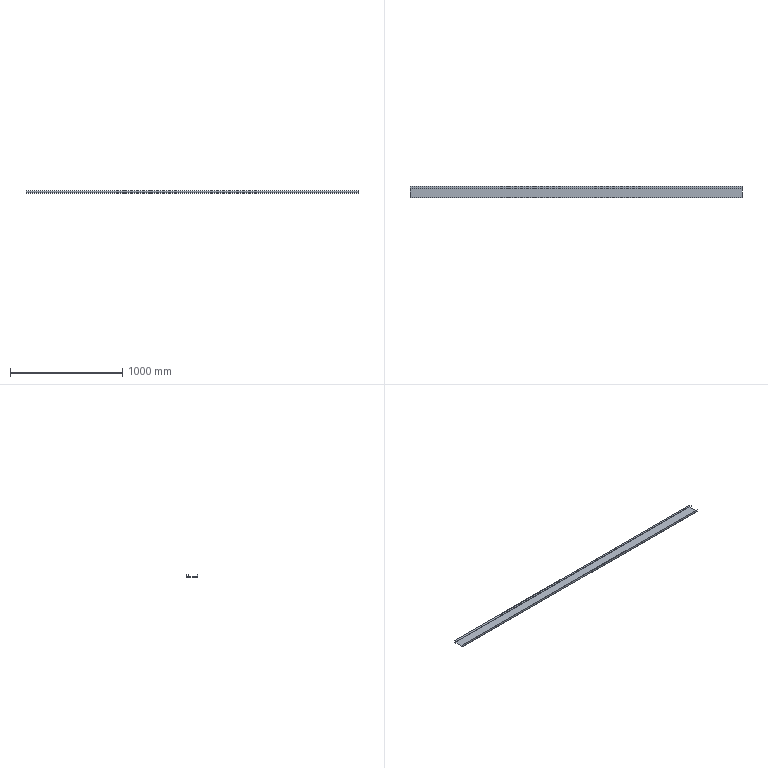Part | STEP file | 粉仓楼梯通道护栏1踢脚Plate | 1 solid | 18 faces | box 2960 x 100 x 20 mm | volume 680415 mm3 | plane 12 | cylinder 6 | commonest cylinder face diameters 2 x3 5 x3
STEP:
#1=CARTESIAN_POINT('',(0.,0.,0.));
#2=DIRECTION('',(0.,0.,1.));
#3=DIRECTION('',(1.,0.,0.));
#4=AXIS2_PLACEMENT_3D('',#1,#2,#3);
#5=CARTESIAN_POINT('',(-1480.,1.5,2.5));
#6=VERTEX_POINT('',#5);
#7=CARTESIAN_POINT('',(-1480.,1.5,20.));
#8=VERTEX_POINT('',#7);
#9=CARTESIAN_POINT('',(-1480.,1.5,2.5));
#10=DIRECTION('',(0.,0.,1.));
#11=VECTOR('',#10,1.);
#12=LINE('',#9,#11);
#13=CARTESIAN_POINT('',(1480.,1.5,2.5));
#14=DIRECTION('',(0.,-1.,0.));
#15=DIRECTION('',(0.,0.,-1.));
#16=AXIS2_PLACEMENT_3D('',#13,#14,#15);
#17=PLANE('',#16);
#18=CARTESIAN_POINT('',(0.,-2960.));
#19=DIRECTION('',(-1.,0.));
#20=VECTOR('',#19,1.);
#21=LINE('',#18,#20);
#22=(GEOMETRIC_REPRESENTATION_CONTEXT(2)PARAMETRIC_REPRESENTATION_CONTEXT()REPRESENTATION_CONTEXT('',''));
#23=DEFINITIONAL_REPRESENTATION('',(#21),#22);
#24=PCURVE('',#17,#23);
#25=CARTESIAN_POINT('',(-1480.,2.5,2.5));
#26=DIRECTION('',(-1.,0.,0.));
#27=DIRECTION('',(0.,0.,1.));
#28=AXIS2_PLACEMENT_3D('',#25,#26,#27);
#29=PLANE('',#28);
#30=CARTESIAN_POINT('',(0.,-1.));
#31=DIRECTION('',(1.,0.));
#32=VECTOR('',#31,1.);
#33=LINE('',#30,#32);
#34=(GEOMETRIC_REPRESENTATION_CONTEXT(2)PARAMETRIC_REPRESENTATION_CONTEXT()REPRESENTATION_CONTEXT('',''));
#35=DEFINITIONAL_REPRESENTATION('',(#33),#34);
#36=PCURVE('',#29,#35);
#37=SURFACE_CURVE('',#12,(#24,#36),.PCURVE_S1.);
#38=EDGE_CURVE('',#6,#8,#37,.T.);
#39=ORIENTED_EDGE('',*,*,#38,.T.);
#40=CARTESIAN_POINT('',(1480.,1.5,20.));
#41=VERTEX_POINT('',#40);
#42=CARTESIAN_POINT('',(1480.,1.5,20.));
#43=DIRECTION('',(-1.,0.,0.));
#44=VECTOR('',#43,1.);
#45=LINE('',#42,#44);
#46=CARTESIAN_POINT('',(-17.5,0.));
#47=DIRECTION('',(0.,-1.));
#48=VECTOR('',#47,1.);
#49=LINE('',#46,#48);
#50=(GEOMETRIC_REPRESENTATION_CONTEXT(2)PARAMETRIC_REPRESENTATION_CONTEXT()REPRESENTATION_CONTEXT('',''));
#51=DEFINITIONAL_REPRESENTATION('',(#49),#50);
#52=PCURVE('',#17,#51);
#53=CARTESIAN_POINT('',(1480.,0.,20.));
#54=DIRECTION('',(0.,0.,1.));
#55=DIRECTION('',(1.,0.,0.));
#56=AXIS2_PLACEMENT_3D('',#53,#54,#55);
#57=PLANE('',#56);
#58=CARTESIAN_POINT('',(0.,1.5));
#59=DIRECTION('',(-1.,0.));
#60=VECTOR('',#59,1.);
#61=LINE('',#58,#60);
#62=(GEOMETRIC_REPRESENTATION_CONTEXT(2)PARAMETRIC_REPRESENTATION_CONTEXT()REPRESENTATION_CONTEXT('',''));
#63=DEFINITIONAL_REPRESENTATION('',(#61),#62);
#64=PCURVE('',#57,#63);
#65=SURFACE_CURVE('',#45,(#52,#64),.PCURVE_S1.);
#66=EDGE_CURVE('',#41,#8,#65,.T.);
#67=ORIENTED_EDGE('',*,*,#66,.F.);
#68=CARTESIAN_POINT('',(1480.,1.5,2.5));
#69=VERTEX_POINT('',#68);
#70=CARTESIAN_POINT('',(1480.,1.5,2.5));
#71=DIRECTION('',(0.,0.,1.));
#72=VECTOR('',#71,1.);
#73=LINE('',#70,#72);
#74=CARTESIAN_POINT('',(0.,0.));
#75=DIRECTION('',(-1.,0.));
#76=VECTOR('',#75,1.);
#77=LINE('',#74,#76);
#78=(GEOMETRIC_REPRESENTATION_CONTEXT(2)PARAMETRIC_REPRESENTATION_CONTEXT()REPRESENTATION_CONTEXT('',''));
#79=DEFINITIONAL_REPRESENTATION('',(#77),#78);
#80=PCURVE('',#17,#79);
#81=CARTESIAN_POINT('',(1480.,2.5,2.5));
#82=DIRECTION('',(-1.,0.,0.));
#83=DIRECTION('',(0.,0.,1.));
#84=AXIS2_PLACEMENT_3D('',#81,#82,#83);
#85=PLANE('',#84);
#86=CARTESIAN_POINT('',(0.,-1.));
#87=DIRECTION('',(1.,0.));
#88=VECTOR('',#87,1.);
#89=LINE('',#86,#88);
#90=(GEOMETRIC_REPRESENTATION_CONTEXT(2)PARAMETRIC_REPRESENTATION_CONTEXT()REPRESENTATION_CONTEXT('',''));
#91=DEFINITIONAL_REPRESENTATION('',(#89),#90);
#92=PCURVE('',#85,#91);
#93=SURFACE_CURVE('',#73,(#80,#92),.PCURVE_S1.);
#94=EDGE_CURVE('',#69,#41,#93,.T.);
#95=ORIENTED_EDGE('',*,*,#94,.F.);
#96=CARTESIAN_POINT('',(1480.,1.5,2.5));
#97=DIRECTION('',(-1.,0.,0.));
#98=VECTOR('',#97,1.);
#99=LINE('',#96,#98);
#100=CARTESIAN_POINT('',(0.,0.));
#101=DIRECTION('',(0.,-1.));
#102=VECTOR('',#101,1.);
#103=LINE('',#100,#102);
#104=(GEOMETRIC_REPRESENTATION_CONTEXT(2)PARAMETRIC_REPRESENTATION_CONTEXT()REPRESENTATION_CONTEXT('',''));
#105=DEFINITIONAL_REPRESENTATION('',(#103),#104);
#106=PCURVE('',#17,#105);
#107=CARTESIAN_POINT('',(1480.,2.5,2.5));
#108=DIRECTION('',(-1.,0.,0.));
#109=DIRECTION('',(0.,0.,1.));
#110=AXIS2_PLACEMENT_3D('',#107,#108,#109);
#111=CYLINDRICAL_SURFACE('',#110,1.);
#112=CARTESIAN_POINT('',(4.712,0.));
#113=DIRECTION('',(0.,1.));
#114=VECTOR('',#113,1.);
#115=LINE('',#112,#114);
#116=(GEOMETRIC_REPRESENTATION_CONTEXT(2)PARAMETRIC_REPRESENTATION_CONTEXT()REPRESENTATION_CONTEXT('',''));
#117=DEFINITIONAL_REPRESENTATION('',(#115),#116);
#118=PCURVE('',#111,#117);
#119=SURFACE_CURVE('',#99,(#106,#118),.PCURVE_S1.);
#120=EDGE_CURVE('',#69,#6,#119,.T.);
#121=ORIENTED_EDGE('',*,*,#120,.T.);
#122=EDGE_LOOP('',(#39,#67,#95,#121));
#123=FACE_BOUND('',#122,.T.);
#124=ADVANCED_FACE('',(#123),#17,.F.);
#125=CARTESIAN_POINT('',(-1480.,0.,20.));
#126=VERTEX_POINT('',#125);
#127=CARTESIAN_POINT('',(-1480.,0.,20.));
#128=DIRECTION('',(0.,1.,0.));
#129=VECTOR('',#128,1.);
#130=LINE('',#127,#129);
#131=CARTESIAN_POINT('',(-2960.,0.));
#132=DIRECTION('',(0.,1.));
#133=VECTOR('',#132,1.);
#134=LINE('',#131,#133);
#135=(GEOMETRIC_REPRESENTATION_CONTEXT(2)PARAMETRIC_REPRESENTATION_CONTEXT()REPRESENTATION_CONTEXT('',''));
#136=DEFINITIONAL_REPRESENTATION('',(#134),#135);
#137=PCURVE('',#57,#136);
#138=CARTESIAN_POINT('',(17.5,-2.5));
#139=DIRECTION('',(0.,1.));
#140=VECTOR('',#139,1.);
#141=LINE('',#138,#140);
#142=(GEOMETRIC_REPRESENTATION_CONTEXT(2)PARAMETRIC_REPRESENTATION_CONTEXT()REPRESENTATION_CONTEXT('',''));
#143=DEFINITIONAL_REPRESENTATION('',(#141),#142);
#144=PCURVE('',#29,#143);
#145=SURFACE_CURVE('',#130,(#137,#144),.PCURVE_S1.);
#146=EDGE_CURVE('',#126,#8,#145,.T.);
#147=ORIENTED_EDGE('',*,*,#146,.F.);
#148=CARTESIAN_POINT('',(1480.,0.,20.));
#149=VERTEX_POINT('',#148);
#150=CARTESIAN_POINT('',(1480.,0.,20.));
#151=DIRECTION('',(-1.,0.,0.));
#152=VECTOR('',#151,1.);
#153=LINE('',#150,#152);
#154=CARTESIAN_POINT('',(0.,0.));
#155=DIRECTION('',(-1.,0.));
#156=VECTOR('',#155,1.);
#157=LINE('',#154,#156);
#158=(GEOMETRIC_REPRESENTATION_CONTEXT(2)PARAMETRIC_REPRESENTATION_CONTEXT()REPRESENTATION_CONTEXT('',''));
#159=DEFINITIONAL_REPRESENTATION('',(#157),#158);
#160=PCURVE('',#57,#159);
#161=CARTESIAN_POINT('',(1480.,0.,2.5));
#162=DIRECTION('',(0.,-1.,0.));
#163=DIRECTION('',(0.,0.,-1.));
#164=AXIS2_PLACEMENT_3D('',#161,#162,#163);
#165=PLANE('',#164);
#166=CARTESIAN_POINT('',(-17.5,0.));
#167=DIRECTION('',(0.,-1.));
#168=VECTOR('',#167,1.);
#169=LINE('',#166,#168);
#170=(GEOMETRIC_REPRESENTATION_CONTEXT(2)PARAMETRIC_REPRESENTATION_CONTEXT()REPRESENTATION_CONTEXT('',''));
#171=DEFINITIONAL_REPRESENTATION('',(#169),#170);
#172=PCURVE('',#165,#171);
#173=SURFACE_CURVE('',#153,(#160,#172),.PCURVE_S1.);
#174=EDGE_CURVE('',#149,#126,#173,.T.);
#175=ORIENTED_EDGE('',*,*,#174,.F.);
#176=CARTESIAN_POINT('',(1480.,0.,20.));
#177=DIRECTION('',(0.,1.,0.));
#178=VECTOR('',#177,1.);
#179=LINE('',#176,#178);
#180=CARTESIAN_POINT('',(0.,0.));
#181=DIRECTION('',(0.,1.));
#182=VECTOR('',#181,1.);
#183=LINE('',#180,#182);
#184=(GEOMETRIC_REPRESENTATION_CONTEXT(2)PARAMETRIC_REPRESENTATION_CONTEXT()REPRESENTATION_CONTEXT('',''));
#185=DEFINITIONAL_REPRESENTATION('',(#183),#184);
#186=PCURVE('',#57,#185);
#187=CARTESIAN_POINT('',(17.5,-2.5));
#188=DIRECTION('',(0.,1.));
#189=VECTOR('',#188,1.);
#190=LINE('',#187,#189);
#191=(GEOMETRIC_REPRESENTATION_CONTEXT(2)PARAMETRIC_REPRESENTATION_CONTEXT()REPRESENTATION_CONTEXT('',''));
#192=DEFINITIONAL_REPRESENTATION('',(#190),#191);
#193=PCURVE('',#85,#192);
#194=SURFACE_CURVE('',#179,(#186,#193),.PCURVE_S1.);
#195=EDGE_CURVE('',#149,#41,#194,.T.);
#196=ORIENTED_EDGE('',*,*,#195,.T.);
#197=ORIENTED_EDGE('',*,*,#66,.T.);
#198=EDGE_LOOP('',(#147,#175,#196,#197));
#199=FACE_BOUND('',#198,.T.);
#200=ADVANCED_FACE('',(#199),#57,.T.);
#201=CARTESIAN_POINT('',(-1480.,0.,2.5));
#202=VERTEX_POINT('',#201);
#203=CARTESIAN_POINT('',(-1480.,0.,2.5));
#204=DIRECTION('',(0.,0.,1.));
#205=VECTOR('',#204,1.);
#206=LINE('',#203,#205);
#207=CARTESIAN_POINT('',(0.,-2960.));
#208=DIRECTION('',(-1.,0.));
#209=VECTOR('',#208,1.);
#210=LINE('',#207,#209);
#211=(GEOMETRIC_REPRESENTATION_CONTEXT(2)PARAMETRIC_REPRESENTATION_CONTEXT()REPRESENTATION_CONTEXT('',''));
#212=DEFINITIONAL_REPRESENTATION('',(#210),#211);
#213=PCURVE('',#165,#212);
#214=CARTESIAN_POINT('',(0.,-2.5));
#215=DIRECTION('',(1.,0.));
#216=VECTOR('',#215,1.);
#217=LINE('',#214,#216);
#218=(GEOMETRIC_REPRESENTATION_CONTEXT(2)PARAMETRIC_REPRESENTATION_CONTEXT()REPRESENTATION_CONTEXT('',''));
#219=DEFINITIONAL_REPRESENTATION('',(#217),#218);
#220=PCURVE('',#29,#219);
#221=SURFACE_CURVE('',#206,(#213,#220),.PCURVE_S1.);
#222=EDGE_CURVE('',#202,#126,#221,.T.);
#223=ORIENTED_EDGE('',*,*,#222,.F.);
#224=CARTESIAN_POINT('',(1480.,0.,2.5));
#225=VERTEX_POINT('',#224);
#226=CARTESIAN_POINT('',(1480.,0.,2.5));
#227=DIRECTION('',(-1.,0.,0.));
#228=VECTOR('',#227,1.);
#229=LINE('',#226,#228);
#230=CARTESIAN_POINT('',(0.,0.));
#231=DIRECTION('',(0.,-1.));
#232=VECTOR('',#231,1.);
#233=LINE('',#230,#232);
#234=(GEOMETRIC_REPRESENTATION_CONTEXT(2)PARAMETRIC_REPRESENTATION_CONTEXT()REPRESENTATION_CONTEXT('',''));
#235=DEFINITIONAL_REPRESENTATION('',(#233),#234);
#236=PCURVE('',#165,#235);
#237=CARTESIAN_POINT('',(1480.,2.5,2.5));
#238=DIRECTION('',(-1.,0.,0.));
#239=DIRECTION('',(0.,0.,1.));
#240=AXIS2_PLACEMENT_3D('',#237,#238,#239);
#241=CYLINDRICAL_SURFACE('',#240,2.5);
#242=CARTESIAN_POINT('',(4.712,0.));
#243=DIRECTION('',(0.,1.));
#244=VECTOR('',#243,1.);
#245=LINE('',#242,#244);
#246=(GEOMETRIC_REPRESENTATION_CONTEXT(2)PARAMETRIC_REPRESENTATION_CONTEXT()REPRESENTATION_CONTEXT('',''));
#247=DEFINITIONAL_REPRESENTATION('',(#245),#246);
#248=PCURVE('',#241,#247);
#249=SURFACE_CURVE('',#229,(#236,#248),.PCURVE_S1.);
#250=EDGE_CURVE('',#225,#202,#249,.T.);
#251=ORIENTED_EDGE('',*,*,#250,.F.);
#252=CARTESIAN_POINT('',(1480.,0.,2.5));
#253=DIRECTION('',(0.,0.,1.));
#254=VECTOR('',#253,1.);
#255=LINE('',#252,#254);
#256=CARTESIAN_POINT('',(0.,0.));
#257=DIRECTION('',(-1.,0.));
#258=VECTOR('',#257,1.);
#259=LINE('',#256,#258);
#260=(GEOMETRIC_REPRESENTATION_CONTEXT(2)PARAMETRIC_REPRESENTATION_CONTEXT()REPRESENTATION_CONTEXT('',''));
#261=DEFINITIONAL_REPRESENTATION('',(#259),#260);
#262=PCURVE('',#165,#261);
#263=CARTESIAN_POINT('',(0.,-2.5));
#264=DIRECTION('',(1.,0.));
#265=VECTOR('',#264,1.);
#266=LINE('',#263,#265);
#267=(GEOMETRIC_REPRESENTATION_CONTEXT(2)PARAMETRIC_REPRESENTATION_CONTEXT()REPRESENTATION_CONTEXT('',''));
#268=DEFINITIONAL_REPRESENTATION('',(#266),#267);
#269=PCURVE('',#85,#268);
#270=SURFACE_CURVE('',#255,(#262,#269),.PCURVE_S1.);
#271=EDGE_CURVE('',#225,#149,#270,.T.);
#272=ORIENTED_EDGE('',*,*,#271,.T.);
#273=ORIENTED_EDGE('',*,*,#174,.T.);
#274=EDGE_LOOP('',(#223,#251,#272,#273));
#275=FACE_BOUND('',#274,.T.);
#276=ADVANCED_FACE('',(#275),#165,.T.);
#277=CARTESIAN_POINT('',(-1480.,2.5,0.));
#278=VERTEX_POINT('',#277);
#279=CARTESIAN_POINT('',(-1480.,2.5,2.5));
#280=DIRECTION('',(-1.,0.,0.));
#281=DIRECTION('',(0.,0.,1.));
#282=AXIS2_PLACEMENT_3D('',#279,#280,#281);
#283=CIRCLE('',#282,2.5);
#284=CARTESIAN_POINT('',(0.,2960.));
#285=DIRECTION('',(1.,0.));
#286=VECTOR('',#285,1.);
#287=LINE('',#284,#286);
#288=(GEOMETRIC_REPRESENTATION_CONTEXT(2)PARAMETRIC_REPRESENTATION_CONTEXT()REPRESENTATION_CONTEXT('',''));
#289=DEFINITIONAL_REPRESENTATION('',(#287),#288);
#290=PCURVE('',#241,#289);
#291=CARTESIAN_POINT('',(0.,0.));
#292=DIRECTION('',(1.,0.));
#293=AXIS2_PLACEMENT_2D('',#291,#292);
#294=CIRCLE('',#293,2.5);
#295=(GEOMETRIC_REPRESENTATION_CONTEXT(2)PARAMETRIC_REPRESENTATION_CONTEXT()REPRESENTATION_CONTEXT('',''));
#296=DEFINITIONAL_REPRESENTATION('',(#294),#295);
#297=PCURVE('',#29,#296);
#298=SURFACE_CURVE('',#283,(#290,#297),.PCURVE_S1.);
#299=EDGE_CURVE('',#278,#202,#298,.T.);
#300=ORIENTED_EDGE('',*,*,#299,.F.);
#301=CARTESIAN_POINT('',(1480.,2.5,0.));
#302=VERTEX_POINT('',#301);
#303=CARTESIAN_POINT('',(1480.,2.5,0.));
#304=DIRECTION('',(-1.,0.,0.));
#305=VECTOR('',#304,1.);
#306=LINE('',#303,#305);
#307=CARTESIAN_POINT('',(3.142,0.));
#308=DIRECTION('',(0.,1.));
#309=VECTOR('',#308,1.);
#310=LINE('',#307,#309);
#311=(GEOMETRIC_REPRESENTATION_CONTEXT(2)PARAMETRIC_REPRESENTATION_CONTEXT()REPRESENTATION_CONTEXT('',''));
#312=DEFINITIONAL_REPRESENTATION('',(#310),#311);
#313=PCURVE('',#241,#312);
#314=CARTESIAN_POINT('',(1480.,2.5,0.));
#315=DIRECTION('',(0.,0.,-1.));
#316=DIRECTION('',(-1.,0.,0.));
#317=AXIS2_PLACEMENT_3D('',#314,#315,#316);
#318=PLANE('',#317);
#319=CARTESIAN_POINT('',(0.,0.));
#320=DIRECTION('',(1.,0.));
#321=VECTOR('',#320,1.);
#322=LINE('',#319,#321);
#323=(GEOMETRIC_REPRESENTATION_CONTEXT(2)PARAMETRIC_REPRESENTATION_CONTEXT()REPRESENTATION_CONTEXT('',''));
#324=DEFINITIONAL_REPRESENTATION('',(#322),#323);
#325=PCURVE('',#318,#324);
#326=SURFACE_CURVE('',#306,(#313,#325),.PCURVE_S1.);
#327=EDGE_CURVE('',#302,#278,#326,.T.);
#328=ORIENTED_EDGE('',*,*,#327,.F.);
#329=CARTESIAN_POINT('',(1480.,2.5,2.5));
#330=DIRECTION('',(-1.,0.,0.));
#331=DIRECTION('',(0.,0.,1.));
#332=AXIS2_PLACEMENT_3D('',#329,#330,#331);
#333=CIRCLE('',#332,2.5);
#334=CARTESIAN_POINT('',(0.,0.));
#335=DIRECTION('',(1.,0.));
#336=VECTOR('',#335,1.);
#337=LINE('',#334,#336);
#338=(GEOMETRIC_REPRESENTATION_CONTEXT(2)PARAMETRIC_REPRESENTATION_CONTEXT()REPRESENTATION_CONTEXT('',''));
#339=DEFINITIONAL_REPRESENTATION('',(#337),#338);
#340=PCURVE('',#241,#339);
#341=CARTESIAN_POINT('',(0.,0.));
#342=DIRECTION('',(1.,0.));
#343=AXIS2_PLACEMENT_2D('',#341,#342);
#344=CIRCLE('',#343,2.5);
#345=(GEOMETRIC_REPRESENTATION_CONTEXT(2)PARAMETRIC_REPRESENTATION_CONTEXT()REPRESENTATION_CONTEXT('',''));
#346=DEFINITIONAL_REPRESENTATION('',(#344),#345);
#347=PCURVE('',#85,#346);
#348=SURFACE_CURVE('',#333,(#340,#347),.PCURVE_S1.);
#349=EDGE_CURVE('',#302,#225,#348,.T.);
#350=ORIENTED_EDGE('',*,*,#349,.T.);
#351=ORIENTED_EDGE('',*,*,#250,.T.);
#352=EDGE_LOOP('',(#300,#328,#350,#351));
#353=FACE_BOUND('',#352,.T.);
#354=ADVANCED_FACE('',(#353),#241,.T.);
#355=CARTESIAN_POINT('',(-1480.,97.5,0.));
#356=VERTEX_POINT('',#355);
#357=CARTESIAN_POINT('',(-1480.,2.5,0.));
#358=DIRECTION('',(0.,-1.,0.));
#359=VECTOR('',#358,1.);
#360=LINE('',#357,#359);
#361=CARTESIAN_POINT('',(2960.,0.));
#362=DIRECTION('',(0.,-1.));
#363=VECTOR('',#362,1.);
#364=LINE('',#361,#363);
#365=(GEOMETRIC_REPRESENTATION_CONTEXT(2)PARAMETRIC_REPRESENTATION_CONTEXT()REPRESENTATION_CONTEXT('',''));
#366=DEFINITIONAL_REPRESENTATION('',(#364),#365);
#367=PCURVE('',#318,#366);
#368=CARTESIAN_POINT('',(-2.5,0.));
#369=DIRECTION('',(0.,-1.));
#370=VECTOR('',#369,1.);
#371=LINE('',#368,#370);
#372=(GEOMETRIC_REPRESENTATION_CONTEXT(2)PARAMETRIC_REPRESENTATION_CONTEXT()REPRESENTATION_CONTEXT('',''));
#373=DEFINITIONAL_REPRESENTATION('',(#371),#372);
#374=PCURVE('',#29,#373);
#375=SURFACE_CURVE('',#360,(#367,#374),.PCURVE_S1.);
#376=EDGE_CURVE('',#356,#278,#375,.T.);
#377=ORIENTED_EDGE('',*,*,#376,.F.);
#378=CARTESIAN_POINT('',(1480.,97.5,0.));
#379=VERTEX_POINT('',#378);
#380=CARTESIAN_POINT('',(1480.,97.5,0.));
#381=DIRECTION('',(-1.,0.,0.));
#382=VECTOR('',#381,1.);
#383=LINE('',#380,#382);
#384=CARTESIAN_POINT('',(0.,95.));
#385=DIRECTION('',(1.,0.));
#386=VECTOR('',#385,1.);
#387=LINE('',#384,#386);
#388=(GEOMETRIC_REPRESENTATION_CONTEXT(2)PARAMETRIC_REPRESENTATION_CONTEXT()REPRESENTATION_CONTEXT('',''));
#389=DEFINITIONAL_REPRESENTATION('',(#387),#388);
#390=PCURVE('',#318,#389);
#391=CARTESIAN_POINT('',(1480.,97.5,2.5));
#392=DIRECTION('',(-1.,0.,0.));
#393=DIRECTION('',(0.,0.,1.));
#394=AXIS2_PLACEMENT_3D('',#391,#392,#393);
#395=CYLINDRICAL_SURFACE('',#394,2.5);
#396=CARTESIAN_POINT('',(3.142,0.));
#397=DIRECTION('',(0.,1.));
#398=VECTOR('',#397,1.);
#399=LINE('',#396,#398);
#400=(GEOMETRIC_REPRESENTATION_CONTEXT(2)PARAMETRIC_REPRESENTATION_CONTEXT()REPRESENTATION_CONTEXT('',''));
#401=DEFINITIONAL_REPRESENTATION('',(#399),#400);
#402=PCURVE('',#395,#401);
#403=SURFACE_CURVE('',#383,(#390,#402),.PCURVE_S1.);
#404=EDGE_CURVE('',#379,#356,#403,.T.);
#405=ORIENTED_EDGE('',*,*,#404,.F.);
#406=CARTESIAN_POINT('',(1480.,2.5,0.));
#407=DIRECTION('',(0.,-1.,0.));
#408=VECTOR('',#407,1.);
#409=LINE('',#406,#408);
#410=CARTESIAN_POINT('',(0.,0.));
#411=DIRECTION('',(0.,-1.));
#412=VECTOR('',#411,1.);
#413=LINE('',#410,#412);
#414=(GEOMETRIC_REPRESENTATION_CONTEXT(2)PARAMETRIC_REPRESENTATION_CONTEXT()REPRESENTATION_CONTEXT('',''));
#415=DEFINITIONAL_REPRESENTATION('',(#413),#414);
#416=PCURVE('',#318,#415);
#417=CARTESIAN_POINT('',(-2.5,0.));
#418=DIRECTION('',(0.,-1.));
#419=VECTOR('',#418,1.);
#420=LINE('',#417,#419);
#421=(GEOMETRIC_REPRESENTATION_CONTEXT(2)PARAMETRIC_REPRESENTATION_CONTEXT()REPRESENTATION_CONTEXT('',''));
#422=DEFINITIONAL_REPRESENTATION('',(#420),#421);
#423=PCURVE('',#85,#422);
#424=SURFACE_CURVE('',#409,(#416,#423),.PCURVE_S1.);
#425=EDGE_CURVE('',#379,#302,#424,.T.);
#426=ORIENTED_EDGE('',*,*,#425,.T.);
#427=ORIENTED_EDGE('',*,*,#327,.T.);
#428=EDGE_LOOP('',(#377,#405,#426,#427));
#429=FACE_BOUND('',#428,.T.);
#430=ADVANCED_FACE('',(#429),#318,.T.);
#431=CARTESIAN_POINT('',(-1480.,100.,2.5));
#432=VERTEX_POINT('',#431);
#433=CARTESIAN_POINT('',(-1480.,97.5,2.5));
#434=DIRECTION('',(-1.,0.,0.));
#435=DIRECTION('',(0.,0.,-1.));
#436=AXIS2_PLACEMENT_3D('',#433,#434,#435);
#437=CIRCLE('',#436,2.5);
#438=CARTESIAN_POINT('',(-3.142,2960.));
#439=DIRECTION('',(1.,0.));
#440=VECTOR('',#439,1.);
#441=LINE('',#438,#440);
#442=(GEOMETRIC_REPRESENTATION_CONTEXT(2)PARAMETRIC_REPRESENTATION_CONTEXT()REPRESENTATION_CONTEXT('',''));
#443=DEFINITIONAL_REPRESENTATION('',(#441),#442);
#444=PCURVE('',#395,#443);
#445=CARTESIAN_POINT('',(0.,95.));
#446=DIRECTION('',(-1.,0.));
#447=AXIS2_PLACEMENT_2D('',#445,#446);
#448=CIRCLE('',#447,2.5);
#449=(GEOMETRIC_REPRESENTATION_CONTEXT(2)PARAMETRIC_REPRESENTATION_CONTEXT()REPRESENTATION_CONTEXT('',''));
#450=DEFINITIONAL_REPRESENTATION('',(#448),#449);
#451=PCURVE('',#29,#450);
#452=SURFACE_CURVE('',#437,(#444,#451),.PCURVE_S1.);
#453=EDGE_CURVE('',#432,#356,#452,.T.);
#454=ORIENTED_EDGE('',*,*,#453,.F.);
#455=CARTESIAN_POINT('',(1480.,100.,2.5));
#456=VERTEX_POINT('',#455);
#457=CARTESIAN_POINT('',(1480.,100.,2.5));
#458=DIRECTION('',(-1.,0.,0.));
#459=VECTOR('',#458,1.);
#460=LINE('',#457,#459);
#461=CARTESIAN_POINT('',(1.571,0.));
#462=DIRECTION('',(0.,1.));
#463=VECTOR('',#462,1.);
#464=LINE('',#461,#463);
#465=(GEOMETRIC_REPRESENTATION_CONTEXT(2)PARAMETRIC_REPRESENTATION_CONTEXT()REPRESENTATION_CONTEXT('',''));
#466=DEFINITIONAL_REPRESENTATION('',(#464),#465);
#467=PCURVE('',#395,#466);
#468=CARTESIAN_POINT('',(1480.,100.,2.5));
#469=DIRECTION('',(0.,1.,0.));
#470=DIRECTION('',(0.,0.,1.));
#471=AXIS2_PLACEMENT_3D('',#468,#469,#470);
#472=PLANE('',#471);
#473=CARTESIAN_POINT('',(0.,0.));
#474=DIRECTION('',(0.,-1.));
#475=VECTOR('',#474,1.);
#476=LINE('',#473,#475);
#477=(GEOMETRIC_REPRESENTATION_CONTEXT(2)PARAMETRIC_REPRESENTATION_CONTEXT()REPRESENTATION_CONTEXT('',''));
#478=DEFINITIONAL_REPRESENTATION('',(#476),#477);
#479=PCURVE('',#472,#478);
#480=SURFACE_CURVE('',#460,(#467,#479),.PCURVE_S1.);
#481=EDGE_CURVE('',#456,#432,#480,.T.);
#482=ORIENTED_EDGE('',*,*,#481,.F.);
#483=CARTESIAN_POINT('',(1480.,97.5,2.5));
#484=DIRECTION('',(-1.,0.,0.));
#485=DIRECTION('',(0.,0.,-1.));
#486=AXIS2_PLACEMENT_3D('',#483,#484,#485);
#487=CIRCLE('',#486,2.5);
#488=CARTESIAN_POINT('',(-3.142,0.));
#489=DIRECTION('',(1.,0.));
#490=VECTOR('',#489,1.);
#491=LINE('',#488,#490);
#492=(GEOMETRIC_REPRESENTATION_CONTEXT(2)PARAMETRIC_REPRESENTATION_CONTEXT()REPRESENTATION_CONTEXT('',''));
#493=DEFINITIONAL_REPRESENTATION('',(#491),#492);
#494=PCURVE('',#395,#493);
#495=CARTESIAN_POINT('',(0.,95.));
#496=DIRECTION('',(-1.,0.));
#497=AXIS2_PLACEMENT_2D('',#495,#496);
#498=CIRCLE('',#497,2.5);
#499=(GEOMETRIC_REPRESENTATION_CONTEXT(2)PARAMETRIC_REPRESENTATION_CONTEXT()REPRESENTATION_CONTEXT('',''));
#500=DEFINITIONAL_REPRESENTATION('',(#498),#499);
#501=PCURVE('',#85,#500);
#502=SURFACE_CURVE('',#487,(#494,#501),.PCURVE_S1.);
#503=EDGE_CURVE('',#456,#379,#502,.T.);
#504=ORIENTED_EDGE('',*,*,#503,.T.);
#505=ORIENTED_EDGE('',*,*,#404,.T.);
#506=EDGE_LOOP('',(#454,#482,#504,#505));
#507=FACE_BOUND('',#506,.T.);
#508=ADVANCED_FACE('',(#507),#395,.T.);
#509=CARTESIAN_POINT('',(-1480.,100.,17.5));
#510=VERTEX_POINT('',#509);
#511=CARTESIAN_POINT('',(-1480.,100.,2.5));
#512=DIRECTION('',(0.,0.,-1.));
#513=VECTOR('',#512,1.);
#514=LINE('',#511,#513);
#515=CARTESIAN_POINT('',(0.,-2960.));
#516=DIRECTION('',(-1.,0.));
#517=VECTOR('',#516,1.);
#518=LINE('',#515,#517);
#519=(GEOMETRIC_REPRESENTATION_CONTEXT(2)PARAMETRIC_REPRESENTATION_CONTEXT()REPRESENTATION_CONTEXT('',''));
#520=DEFINITIONAL_REPRESENTATION('',(#518),#519);
#521=PCURVE('',#472,#520);
#522=CARTESIAN_POINT('',(0.,97.5));
#523=DIRECTION('',(-1.,0.));
#524=VECTOR('',#523,1.);
#525=LINE('',#522,#524);
#526=(GEOMETRIC_REPRESENTATION_CONTEXT(2)PARAMETRIC_REPRESENTATION_CONTEXT()REPRESENTATION_CONTEXT('',''));
#527=DEFINITIONAL_REPRESENTATION('',(#525),#526);
#528=PCURVE('',#29,#527);
#529=SURFACE_CURVE('',#514,(#521,#528),.PCURVE_S1.);
#530=EDGE_CURVE('',#510,#432,#529,.T.);
#531=ORIENTED_EDGE('',*,*,#530,.F.);
#532=CARTESIAN_POINT('',(1480.,100.,17.5));
#533=VERTEX_POINT('',#532);
#534=CARTESIAN_POINT('',(1480.,100.,17.5));
#535=DIRECTION('',(-1.,0.,0.));
#536=VECTOR('',#535,1.);
#537=LINE('',#534,#536);
#538=CARTESIAN_POINT('',(15.,0.));
#539=DIRECTION('',(0.,-1.));
#540=VECTOR('',#539,1.);
#541=LINE('',#538,#540);
#542=(GEOMETRIC_REPRESENTATION_CONTEXT(2)PARAMETRIC_REPRESENTATION_CONTEXT()REPRESENTATION_CONTEXT('',''));
#543=DEFINITIONAL_REPRESENTATION('',(#541),#542);
#544=PCURVE('',#472,#543);
#545=CARTESIAN_POINT('',(1480.,97.5,17.5));
#546=DIRECTION('',(-1.,0.,0.));
#547=DIRECTION('',(0.,0.,1.));
#548=AXIS2_PLACEMENT_3D('',#545,#546,#547);
#549=CYLINDRICAL_SURFACE('',#548,2.5);
#550=CARTESIAN_POINT('',(1.571,0.));
#551=DIRECTION('',(0.,1.));
#552=VECTOR('',#551,1.);
#553=LINE('',#550,#552);
#554=(GEOMETRIC_REPRESENTATION_CONTEXT(2)PARAMETRIC_REPRESENTATION_CONTEXT()REPRESENTATION_CONTEXT('',''));
#555=DEFINITIONAL_REPRESENTATION('',(#553),#554);
#556=PCURVE('',#549,#555);
#557=SURFACE_CURVE('',#537,(#544,#556),.PCURVE_S1.);
#558=EDGE_CURVE('',#533,#510,#557,.T.);
#559=ORIENTED_EDGE('',*,*,#558,.F.);
#560=CARTESIAN_POINT('',(1480.,100.,2.5));
#561=DIRECTION('',(0.,0.,-1.));
#562=VECTOR('',#561,1.);
#563=LINE('',#560,#562);
#564=CARTESIAN_POINT('',(0.,0.));
#565=DIRECTION('',(-1.,0.));
#566=VECTOR('',#565,1.);
#567=LINE('',#564,#566);
#568=(GEOMETRIC_REPRESENTATION_CONTEXT(2)PARAMETRIC_REPRESENTATION_CONTEXT()REPRESENTATION_CONTEXT('',''));
#569=DEFINITIONAL_REPRESENTATION('',(#567),#568);
#570=PCURVE('',#472,#569);
#571=CARTESIAN_POINT('',(0.,97.5));
#572=DIRECTION('',(-1.,0.));
#573=VECTOR('',#572,1.);
#574=LINE('',#571,#573);
#575=(GEOMETRIC_REPRESENTATION_CONTEXT(2)PARAMETRIC_REPRESENTATION_CONTEXT()REPRESENTATION_CONTEXT('',''));
#576=DEFINITIONAL_REPRESENTATION('',(#574),#575);
#577=PCURVE('',#85,#576);
#578=SURFACE_CURVE('',#563,(#570,#577),.PCURVE_S1.);
#579=EDGE_CURVE('',#533,#456,#578,.T.);
#580=ORIENTED_EDGE('',*,*,#579,.T.);
#581=ORIENTED_EDGE('',*,*,#481,.T.);
#582=EDGE_LOOP('',(#531,#559,#580,#581));
#583=FACE_BOUND('',#582,.T.);
#584=ADVANCED_FACE('',(#583),#472,.T.);
#585=CARTESIAN_POINT('',(-1480.,97.5,20.));
#586=VERTEX_POINT('',#585);
#587=CARTESIAN_POINT('',(-1480.,97.5,17.5));
#588=DIRECTION('',(-1.,0.,0.));
#589=DIRECTION('',(0.,0.,-1.));
#590=AXIS2_PLACEMENT_3D('',#587,#588,#589);
#591=CIRCLE('',#590,2.5);
#592=CARTESIAN_POINT('',(-3.142,2960.));
#593=DIRECTION('',(1.,0.));
#594=VECTOR('',#593,1.);
#595=LINE('',#592,#594);
#596=(GEOMETRIC_REPRESENTATION_CONTEXT(2)PARAMETRIC_REPRESENTATION_CONTEXT()REPRESENTATION_CONTEXT('',''));
#597=DEFINITIONAL_REPRESENTATION('',(#595),#596);
#598=PCURVE('',#549,#597);
#599=CARTESIAN_POINT('',(15.,95.));
#600=DIRECTION('',(-1.,0.));
#601=AXIS2_PLACEMENT_2D('',#599,#600);
#602=CIRCLE('',#601,2.5);
#603=(GEOMETRIC_REPRESENTATION_CONTEXT(2)PARAMETRIC_REPRESENTATION_CONTEXT()REPRESENTATION_CONTEXT('',''));
#604=DEFINITIONAL_REPRESENTATION('',(#602),#603);
#605=PCURVE('',#29,#604);
#606=SURFACE_CURVE('',#591,(#598,#605),.PCURVE_S1.);
#607=EDGE_CURVE('',#586,#510,#606,.T.);
#608=ORIENTED_EDGE('',*,*,#607,.F.);
#609=CARTESIAN_POINT('',(1480.,97.5,20.));
#610=VERTEX_POINT('',#609);
#611=CARTESIAN_POINT('',(1480.,97.5,20.));
#612=DIRECTION('',(-1.,0.,0.));
#613=VECTOR('',#612,1.);
#614=LINE('',#611,#613);
#615=CARTESIAN_POINT('',(0.,0.));
#616=DIRECTION('',(0.,1.));
#617=VECTOR('',#616,1.);
#618=LINE('',#615,#617);
#619=(GEOMETRIC_REPRESENTATION_CONTEXT(2)PARAMETRIC_REPRESENTATION_CONTEXT()REPRESENTATION_CONTEXT('',''));
#620=DEFINITIONAL_REPRESENTATION('',(#618),#619);
#621=PCURVE('',#549,#620);
#622=CARTESIAN_POINT('',(1480.,97.5,20.));
#623=DIRECTION('',(0.,0.,1.));
#624=DIRECTION('',(1.,0.,0.));
#625=AXIS2_PLACEMENT_3D('',#622,#623,#624);
#626=PLANE('',#625);
#627=CARTESIAN_POINT('',(0.,0.));
#628=DIRECTION('',(-1.,0.));
#629=VECTOR('',#628,1.);
#630=LINE('',#627,#629);
#631=(GEOMETRIC_REPRESENTATION_CONTEXT(2)PARAMETRIC_REPRESENTATION_CONTEXT()REPRESENTATION_CONTEXT('',''));
#632=DEFINITIONAL_REPRESENTATION('',(#630),#631);
#633=PCURVE('',#626,#632);
#634=SURFACE_CURVE('',#614,(#621,#633),.PCURVE_S1.);
#635=EDGE_CURVE('',#610,#586,#634,.T.);
#636=ORIENTED_EDGE('',*,*,#635,.F.);
#637=CARTESIAN_POINT('',(1480.,97.5,17.5));
#638=DIRECTION('',(-1.,0.,0.));
#639=DIRECTION('',(0.,0.,-1.));
#640=AXIS2_PLACEMENT_3D('',#637,#638,#639);
#641=CIRCLE('',#640,2.5);
#642=CARTESIAN_POINT('',(-3.142,0.));
#643=DIRECTION('',(1.,0.));
#644=VECTOR('',#643,1.);
#645=LINE('',#642,#644);
#646=(GEOMETRIC_REPRESENTATION_CONTEXT(2)PARAMETRIC_REPRESENTATION_CONTEXT()REPRESENTATION_CONTEXT('',''));
#647=DEFINITIONAL_REPRESENTATION('',(#645),#646);
#648=PCURVE('',#549,#647);
#649=CARTESIAN_POINT('',(15.,95.));
#650=DIRECTION('',(-1.,0.));
#651=AXIS2_PLACEMENT_2D('',#649,#650);
#652=CIRCLE('',#651,2.5);
#653=(GEOMETRIC_REPRESENTATION_CONTEXT(2)PARAMETRIC_REPRESENTATION_CONTEXT()REPRESENTATION_CONTEXT('',''));
#654=DEFINITIONAL_REPRESENTATION('',(#652),#653);
#655=PCURVE('',#85,#654);
#656=SURFACE_CURVE('',#641,(#648,#655),.PCURVE_S1.);
#657=EDGE_CURVE('',#610,#533,#656,.T.);
#658=ORIENTED_EDGE('',*,*,#657,.T.);
#659=ORIENTED_EDGE('',*,*,#558,.T.);
#660=EDGE_LOOP('',(#608,#636,#658,#659));
#661=FACE_BOUND('',#660,.T.);
#662=ADVANCED_FACE('',(#661),#549,.T.);
#663=CARTESIAN_POINT('',(-1480.,80.,20.));
#664=VERTEX_POINT('',#663);
#665=CARTESIAN_POINT('',(-1480.,97.5,20.));
#666=DIRECTION('',(0.,1.,0.));
#667=VECTOR('',#666,1.);
#668=LINE('',#665,#667);
#669=CARTESIAN_POINT('',(-2960.,0.));
#670=DIRECTION('',(0.,1.));
#671=VECTOR('',#670,1.);
#672=LINE('',#669,#671);
#673=(GEOMETRIC_REPRESENTATION_CONTEXT(2)PARAMETRIC_REPRESENTATION_CONTEXT()REPRESENTATION_CONTEXT('',''));
#674=DEFINITIONAL_REPRESENTATION('',(#672),#673);
#675=PCURVE('',#626,#674);
#676=CARTESIAN_POINT('',(17.5,95.));
#677=DIRECTION('',(0.,1.));
#678=VECTOR('',#677,1.);
#679=LINE('',#676,#678);
#680=(GEOMETRIC_REPRESENTATION_CONTEXT(2)PARAMETRIC_REPRESENTATION_CONTEXT()REPRESENTATION_CONTEXT('',''));
#681=DEFINITIONAL_REPRESENTATION('',(#679),#680);
#682=PCURVE('',#29,#681);
#683=SURFACE_CURVE('',#668,(#675,#682),.PCURVE_S1.);
#684=EDGE_CURVE('',#664,#586,#683,.T.);
#685=ORIENTED_EDGE('',*,*,#684,.F.);
#686=CARTESIAN_POINT('',(1480.,80.,20.));
#687=VERTEX_POINT('',#686);
#688=CARTESIAN_POINT('',(1480.,80.,20.));
#689=DIRECTION('',(-1.,0.,0.));
#690=VECTOR('',#689,1.);
#691=LINE('',#688,#690);
#692=CARTESIAN_POINT('',(0.,-17.5));
#693=DIRECTION('',(-1.,0.));
#694=VECTOR('',#693,1.);
#695=LINE('',#692,#694);
#696=(GEOMETRIC_REPRESENTATION_CONTEXT(2)PARAMETRIC_REPRESENTATION_CONTEXT()REPRESENTATION_CONTEXT('',''));
#697=DEFINITIONAL_REPRESENTATION('',(#695),#696);
#698=PCURVE('',#626,#697);
#699=CARTESIAN_POINT('',(1480.,80.,18.5));
#700=DIRECTION('',(0.,-1.,0.));
#701=DIRECTION('',(0.,0.,-1.));
#702=AXIS2_PLACEMENT_3D('',#699,#700,#701);
#703=PLANE('',#702);
#704=CARTESIAN_POINT('',(-1.5,0.));
#705=DIRECTION('',(0.,-1.));
#706=VECTOR('',#705,1.);
#707=LINE('',#704,#706);
#708=(GEOMETRIC_REPRESENTATION_CONTEXT(2)PARAMETRIC_REPRESENTATION_CONTEXT()REPRESENTATION_CONTEXT('',''));
#709=DEFINITIONAL_REPRESENTATION('',(#707),#708);
#710=PCURVE('',#703,#709);
#711=SURFACE_CURVE('',#691,(#698,#710),.PCURVE_S1.);
#712=EDGE_CURVE('',#687,#664,#711,.T.);
#713=ORIENTED_EDGE('',*,*,#712,.F.);
#714=CARTESIAN_POINT('',(1480.,97.5,20.));
#715=DIRECTION('',(0.,1.,0.));
#716=VECTOR('',#715,1.);
#717=LINE('',#714,#716);
#718=CARTESIAN_POINT('',(0.,0.));
#719=DIRECTION('',(0.,1.));
#720=VECTOR('',#719,1.);
#721=LINE('',#718,#720);
#722=(GEOMETRIC_REPRESENTATION_CONTEXT(2)PARAMETRIC_REPRESENTATION_CONTEXT()REPRESENTATION_CONTEXT('',''));
#723=DEFINITIONAL_REPRESENTATION('',(#721),#722);
#724=PCURVE('',#626,#723);
#725=CARTESIAN_POINT('',(17.5,95.));
#726=DIRECTION('',(0.,1.));
#727=VECTOR('',#726,1.);
#728=LINE('',#725,#727);
#729=(GEOMETRIC_REPRESENTATION_CONTEXT(2)PARAMETRIC_REPRESENTATION_CONTEXT()REPRESENTATION_CONTEXT('',''));
#730=DEFINITIONAL_REPRESENTATION('',(#728),#729);
#731=PCURVE('',#85,#730);
#732=SURFACE_CURVE('',#717,(#724,#731),.PCURVE_S1.);
#733=EDGE_CURVE('',#687,#610,#732,.T.);
#734=ORIENTED_EDGE('',*,*,#733,.T.);
#735=ORIENTED_EDGE('',*,*,#635,.T.);
#736=EDGE_LOOP('',(#685,#713,#734,#735));
#737=FACE_BOUND('',#736,.T.);
#738=ADVANCED_FACE('',(#737),#626,.T.);
#739=CARTESIAN_POINT('',(-1480.,80.,18.5));
#740=VERTEX_POINT('',#739);
#741=CARTESIAN_POINT('',(-1480.,80.,18.5));
#742=DIRECTION('',(0.,0.,1.));
#743=VECTOR('',#742,1.);
#744=LINE('',#741,#743);
#745=CARTESIAN_POINT('',(0.,-2960.));
#746=DIRECTION('',(-1.,0.));
#747=VECTOR('',#746,1.);
#748=LINE('',#745,#747);
#749=(GEOMETRIC_REPRESENTATION_CONTEXT(2)PARAMETRIC_REPRESENTATION_CONTEXT()REPRESENTATION_CONTEXT('',''));
#750=DEFINITIONAL_REPRESENTATION('',(#748),#749);
#751=PCURVE('',#703,#750);
#752=CARTESIAN_POINT('',(16.,77.5));
#753=DIRECTION('',(1.,0.));
#754=VECTOR('',#753,1.);
#755=LINE('',#752,#754);
#756=(GEOMETRIC_REPRESENTATION_CONTEXT(2)PARAMETRIC_REPRESENTATION_CONTEXT()REPRESENTATION_CONTEXT('',''));
#757=DEFINITIONAL_REPRESENTATION('',(#755),#756);
#758=PCURVE('',#29,#757);
#759=SURFACE_CURVE('',#744,(#751,#758),.PCURVE_S1.);
#760=EDGE_CURVE('',#740,#664,#759,.T.);
#761=ORIENTED_EDGE('',*,*,#760,.F.);
#762=CARTESIAN_POINT('',(1480.,80.,18.5));
#763=VERTEX_POINT('',#762);
#764=CARTESIAN_POINT('',(1480.,80.,18.5));
#765=DIRECTION('',(-1.,0.,0.));
#766=VECTOR('',#765,1.);
#767=LINE('',#764,#766);
#768=CARTESIAN_POINT('',(0.,0.));
#769=DIRECTION('',(0.,-1.));
#770=VECTOR('',#769,1.);
#771=LINE('',#768,#770);
#772=(GEOMETRIC_REPRESENTATION_CONTEXT(2)PARAMETRIC_REPRESENTATION_CONTEXT()REPRESENTATION_CONTEXT('',''));
#773=DEFINITIONAL_REPRESENTATION('',(#771),#772);
#774=PCURVE('',#703,#773);
#775=CARTESIAN_POINT('',(1480.,97.5,18.5));
#776=DIRECTION('',(0.,0.,1.));
#777=DIRECTION('',(1.,0.,0.));
#778=AXIS2_PLACEMENT_3D('',#775,#776,#777);
#779=PLANE('',#778);
#780=CARTESIAN_POINT('',(0.,-17.5));
#781=DIRECTION('',(-1.,0.));
#782=VECTOR('',#781,1.);
#783=LINE('',#780,#782);
#784=(GEOMETRIC_REPRESENTATION_CONTEXT(2)PARAMETRIC_REPRESENTATION_CONTEXT()REPRESENTATION_CONTEXT('',''));
#785=DEFINITIONAL_REPRESENTATION('',(#783),#784);
#786=PCURVE('',#779,#785);
#787=SURFACE_CURVE('',#767,(#774,#786),.PCURVE_S1.);
#788=EDGE_CURVE('',#763,#740,#787,.T.);
#789=ORIENTED_EDGE('',*,*,#788,.F.);
#790=CARTESIAN_POINT('',(1480.,80.,18.5));
#791=DIRECTION('',(0.,0.,1.));
#792=VECTOR('',#791,1.);
#793=LINE('',#790,#792);
#794=CARTESIAN_POINT('',(0.,0.));
#795=DIRECTION('',(-1.,0.));
#796=VECTOR('',#795,1.);
#797=LINE('',#794,#796);
#798=(GEOMETRIC_REPRESENTATION_CONTEXT(2)PARAMETRIC_REPRESENTATION_CONTEXT()REPRESENTATION_CONTEXT('',''));
#799=DEFINITIONAL_REPRESENTATION('',(#797),#798);
#800=PCURVE('',#703,#799);
#801=CARTESIAN_POINT('',(16.,77.5));
#802=DIRECTION('',(1.,0.));
#803=VECTOR('',#802,1.);
#804=LINE('',#801,#803);
#805=(GEOMETRIC_REPRESENTATION_CONTEXT(2)PARAMETRIC_REPRESENTATION_CONTEXT()REPRESENTATION_CONTEXT('',''));
#806=DEFINITIONAL_REPRESENTATION('',(#804),#805);
#807=PCURVE('',#85,#806);
#808=SURFACE_CURVE('',#793,(#800,#807),.PCURVE_S1.);
#809=EDGE_CURVE('',#763,#687,#808,.T.);
#810=ORIENTED_EDGE('',*,*,#809,.T.);
#811=ORIENTED_EDGE('',*,*,#712,.T.);
#812=EDGE_LOOP('',(#761,#789,#810,#811));
#813=FACE_BOUND('',#812,.T.);
#814=ADVANCED_FACE('',(#813),#703,.T.);
#815=CARTESIAN_POINT('',(-1480.,97.5,18.5));
#816=VERTEX_POINT('',#815);
#817=CARTESIAN_POINT('',(-1480.,97.5,18.5));
#818=DIRECTION('',(0.,1.,0.));
#819=VECTOR('',#818,1.);
#820=LINE('',#817,#819);
#821=CARTESIAN_POINT('',(-2960.,0.));
#822=DIRECTION('',(0.,1.));
#823=VECTOR('',#822,1.);
#824=LINE('',#821,#823);
#825=(GEOMETRIC_REPRESENTATION_CONTEXT(2)PARAMETRIC_REPRESENTATION_CONTEXT()REPRESENTATION_CONTEXT('',''));
#826=DEFINITIONAL_REPRESENTATION('',(#824),#825);
#827=PCURVE('',#779,#826);
#828=CARTESIAN_POINT('',(16.,95.));
#829=DIRECTION('',(0.,1.));
#830=VECTOR('',#829,1.);
#831=LINE('',#828,#830);
#832=(GEOMETRIC_REPRESENTATION_CONTEXT(2)PARAMETRIC_REPRESENTATION_CONTEXT()REPRESENTATION_CONTEXT('',''));
#833=DEFINITIONAL_REPRESENTATION('',(#831),#832);
#834=PCURVE('',#29,#833);
#835=SURFACE_CURVE('',#820,(#827,#834),.PCURVE_S1.);
#836=EDGE_CURVE('',#740,#816,#835,.T.);
#837=ORIENTED_EDGE('',*,*,#836,.T.);
#838=CARTESIAN_POINT('',(1480.,97.5,18.5));
#839=VERTEX_POINT('',#838);
#840=CARTESIAN_POINT('',(1480.,97.5,18.5));
#841=DIRECTION('',(-1.,0.,0.));
#842=VECTOR('',#841,1.);
#843=LINE('',#840,#842);
#844=CARTESIAN_POINT('',(0.,0.));
#845=DIRECTION('',(-1.,0.));
#846=VECTOR('',#845,1.);
#847=LINE('',#844,#846);
#848=(GEOMETRIC_REPRESENTATION_CONTEXT(2)PARAMETRIC_REPRESENTATION_CONTEXT()REPRESENTATION_CONTEXT('',''));
#849=DEFINITIONAL_REPRESENTATION('',(#847),#848);
#850=PCURVE('',#779,#849);
#851=CARTESIAN_POINT('',(1480.,97.5,17.5));
#852=DIRECTION('',(-1.,0.,0.));
#853=DIRECTION('',(0.,0.,1.));
#854=AXIS2_PLACEMENT_3D('',#851,#852,#853);
#855=CYLINDRICAL_SURFACE('',#854,1.);
#856=CARTESIAN_POINT('',(0.,0.));
#857=DIRECTION('',(0.,1.));
#858=VECTOR('',#857,1.);
#859=LINE('',#856,#858);
#860=(GEOMETRIC_REPRESENTATION_CONTEXT(2)PARAMETRIC_REPRESENTATION_CONTEXT()REPRESENTATION_CONTEXT('',''));
#861=DEFINITIONAL_REPRESENTATION('',(#859),#860);
#862=PCURVE('',#855,#861);
#863=SURFACE_CURVE('',#843,(#850,#862),.PCURVE_S1.);
#864=EDGE_CURVE('',#839,#816,#863,.T.);
#865=ORIENTED_EDGE('',*,*,#864,.F.);
#866=CARTESIAN_POINT('',(1480.,97.5,18.5));
#867=DIRECTION('',(0.,1.,0.));
#868=VECTOR('',#867,1.);
#869=LINE('',#866,#868);
#870=CARTESIAN_POINT('',(0.,0.));
#871=DIRECTION('',(0.,1.));
#872=VECTOR('',#871,1.);
#873=LINE('',#870,#872);
#874=(GEOMETRIC_REPRESENTATION_CONTEXT(2)PARAMETRIC_REPRESENTATION_CONTEXT()REPRESENTATION_CONTEXT('',''));
#875=DEFINITIONAL_REPRESENTATION('',(#873),#874);
#876=PCURVE('',#779,#875);
#877=CARTESIAN_POINT('',(16.,95.));
#878=DIRECTION('',(0.,1.));
#879=VECTOR('',#878,1.);
#880=LINE('',#877,#879);
#881=(GEOMETRIC_REPRESENTATION_CONTEXT(2)PARAMETRIC_REPRESENTATION_CONTEXT()REPRESENTATION_CONTEXT('',''));
#882=DEFINITIONAL_REPRESENTATION('',(#880),#881);
#883=PCURVE('',#85,#882);
#884=SURFACE_CURVE('',#869,(#876,#883),.PCURVE_S1.);
#885=EDGE_CURVE('',#763,#839,#884,.T.);
#886=ORIENTED_EDGE('',*,*,#885,.F.);
#887=ORIENTED_EDGE('',*,*,#788,.T.);
#888=EDGE_LOOP('',(#837,#865,#886,#887));
#889=FACE_BOUND('',#888,.T.);
#890=ADVANCED_FACE('',(#889),#779,.F.);
#891=ORIENTED_EDGE('',*,*,#864,.F.);
#892=CARTESIAN_POINT('',(1480.,98.5,17.5));
#893=VERTEX_POINT('',#892);
#894=CARTESIAN_POINT('',(1480.,97.5,17.5));
#895=DIRECTION('',(-1.,0.,0.));
#896=DIRECTION('',(0.,0.,-1.));
#897=AXIS2_PLACEMENT_3D('',#894,#895,#896);
#898=CIRCLE('',#897,1.);
#899=CARTESIAN_POINT('',(-3.142,0.));
#900=DIRECTION('',(1.,0.));
#901=VECTOR('',#900,1.);
#902=LINE('',#899,#901);
#903=(GEOMETRIC_REPRESENTATION_CONTEXT(2)PARAMETRIC_REPRESENTATION_CONTEXT()REPRESENTATION_CONTEXT('',''));
#904=DEFINITIONAL_REPRESENTATION('',(#902),#903);
#905=PCURVE('',#855,#904);
#906=CARTESIAN_POINT('',(15.,95.));
#907=DIRECTION('',(-1.,0.));
#908=AXIS2_PLACEMENT_2D('',#906,#907);
#909=CIRCLE('',#908,1.);
#910=(GEOMETRIC_REPRESENTATION_CONTEXT(2)PARAMETRIC_REPRESENTATION_CONTEXT()REPRESENTATION_CONTEXT('',''));
#911=DEFINITIONAL_REPRESENTATION('',(#909),#910);
#912=PCURVE('',#85,#911);
#913=SURFACE_CURVE('',#898,(#905,#912),.PCURVE_S1.);
#914=EDGE_CURVE('',#839,#893,#913,.T.);
#915=ORIENTED_EDGE('',*,*,#914,.T.);
#916=CARTESIAN_POINT('',(-1480.,98.5,17.5));
#917=VERTEX_POINT('',#916);
#918=CARTESIAN_POINT('',(1480.,98.5,17.5));
#919=DIRECTION('',(-1.,0.,0.));
#920=VECTOR('',#919,1.);
#921=LINE('',#918,#920);
#922=CARTESIAN_POINT('',(1.571,0.));
#923=DIRECTION('',(0.,1.));
#924=VECTOR('',#923,1.);
#925=LINE('',#922,#924);
#926=(GEOMETRIC_REPRESENTATION_CONTEXT(2)PARAMETRIC_REPRESENTATION_CONTEXT()REPRESENTATION_CONTEXT('',''));
#927=DEFINITIONAL_REPRESENTATION('',(#925),#926);
#928=PCURVE('',#855,#927);
#929=CARTESIAN_POINT('',(1480.,98.5,2.5));
#930=DIRECTION('',(0.,1.,0.));
#931=DIRECTION('',(0.,0.,1.));
#932=AXIS2_PLACEMENT_3D('',#929,#930,#931);
#933=PLANE('',#932);
#934=CARTESIAN_POINT('',(15.,0.));
#935=DIRECTION('',(0.,-1.));
#936=VECTOR('',#935,1.);
#937=LINE('',#934,#936);
#938=(GEOMETRIC_REPRESENTATION_CONTEXT(2)PARAMETRIC_REPRESENTATION_CONTEXT()REPRESENTATION_CONTEXT('',''));
#939=DEFINITIONAL_REPRESENTATION('',(#937),#938);
#940=PCURVE('',#933,#939);
#941=SURFACE_CURVE('',#921,(#928,#940),.PCURVE_S1.);
#942=EDGE_CURVE('',#893,#917,#941,.T.);
#943=ORIENTED_EDGE('',*,*,#942,.T.);
#944=CARTESIAN_POINT('',(-1480.,97.5,17.5));
#945=DIRECTION('',(-1.,0.,0.));
#946=DIRECTION('',(0.,0.,-1.));
#947=AXIS2_PLACEMENT_3D('',#944,#945,#946);
#948=CIRCLE('',#947,1.);
#949=CARTESIAN_POINT('',(-3.142,2960.));
#950=DIRECTION('',(1.,0.));
#951=VECTOR('',#950,1.);
#952=LINE('',#949,#951);
#953=(GEOMETRIC_REPRESENTATION_CONTEXT(2)PARAMETRIC_REPRESENTATION_CONTEXT()REPRESENTATION_CONTEXT('',''));
#954=DEFINITIONAL_REPRESENTATION('',(#952),#953);
#955=PCURVE('',#855,#954);
#956=CARTESIAN_POINT('',(15.,95.));
#957=DIRECTION('',(-1.,0.));
#958=AXIS2_PLACEMENT_2D('',#956,#957);
#959=CIRCLE('',#958,1.);
#960=(GEOMETRIC_REPRESENTATION_CONTEXT(2)PARAMETRIC_REPRESENTATION_CONTEXT()REPRESENTATION_CONTEXT('',''));
#961=DEFINITIONAL_REPRESENTATION('',(#959),#960);
#962=PCURVE('',#29,#961);
#963=SURFACE_CURVE('',#948,(#955,#962),.PCURVE_S1.);
#964=EDGE_CURVE('',#816,#917,#963,.T.);
#965=ORIENTED_EDGE('',*,*,#964,.F.);
#966=EDGE_LOOP('',(#891,#915,#943,#965));
#967=FACE_BOUND('',#966,.F.);
#968=ADVANCED_FACE('',(#967),#855,.F.);
#969=CARTESIAN_POINT('',(-1480.,98.5,2.5));
#970=VERTEX_POINT('',#969);
#971=CARTESIAN_POINT('',(-1480.,98.5,2.5));
#972=DIRECTION('',(0.,0.,-1.));
#973=VECTOR('',#972,1.);
#974=LINE('',#971,#973);
#975=CARTESIAN_POINT('',(0.,-2960.));
#976=DIRECTION('',(-1.,0.));
#977=VECTOR('',#976,1.);
#978=LINE('',#975,#977);
#979=(GEOMETRIC_REPRESENTATION_CONTEXT(2)PARAMETRIC_REPRESENTATION_CONTEXT()REPRESENTATION_CONTEXT('',''));
#980=DEFINITIONAL_REPRESENTATION('',(#978),#979);
#981=PCURVE('',#933,#980);
#982=CARTESIAN_POINT('',(0.,96.));
#983=DIRECTION('',(-1.,0.));
#984=VECTOR('',#983,1.);
#985=LINE('',#982,#984);
#986=(GEOMETRIC_REPRESENTATION_CONTEXT(2)PARAMETRIC_REPRESENTATION_CONTEXT()REPRESENTATION_CONTEXT('',''));
#987=DEFINITIONAL_REPRESENTATION('',(#985),#986);
#988=PCURVE('',#29,#987);
#989=SURFACE_CURVE('',#974,(#981,#988),.PCURVE_S1.);
#990=EDGE_CURVE('',#917,#970,#989,.T.);
#991=ORIENTED_EDGE('',*,*,#990,.T.);
#992=CARTESIAN_POINT('',(1480.,98.5,2.5));
#993=VERTEX_POINT('',#992);
#994=CARTESIAN_POINT('',(1480.,98.5,2.5));
#995=DIRECTION('',(-1.,0.,0.));
#996=VECTOR('',#995,1.);
#997=LINE('',#994,#996);
#998=CARTESIAN_POINT('',(0.,0.));
#999=DIRECTION('',(0.,-1.));
#1000=VECTOR('',#999,1.);
#1001=LINE('',#998,#1000);
#1002=(GEOMETRIC_REPRESENTATION_CONTEXT(2)PARAMETRIC_REPRESENTATION_CONTEXT()REPRESENTATION_CONTEXT('',''));
#1003=DEFINITIONAL_REPRESENTATION('',(#1001),#1002);
#1004=PCURVE('',#933,#1003);
#1005=CARTESIAN_POINT('',(1480.,97.5,2.5));
#1006=DIRECTION('',(-1.,0.,0.));
#1007=DIRECTION('',(0.,0.,1.));
#1008=AXIS2_PLACEMENT_3D('',#1005,#1006,#1007);
#1009=CYLINDRICAL_SURFACE('',#1008,1.);
#1010=CARTESIAN_POINT('',(1.571,0.));
#1011=DIRECTION('',(0.,1.));
#1012=VECTOR('',#1011,1.);
#1013=LINE('',#1010,#1012);
#1014=(GEOMETRIC_REPRESENTATION_CONTEXT(2)PARAMETRIC_REPRESENTATION_CONTEXT()REPRESENTATION_CONTEXT('',''));
#1015=DEFINITIONAL_REPRESENTATION('',(#1013),#1014);
#1016=PCURVE('',#1009,#1015);
#1017=SURFACE_CURVE('',#997,(#1004,#1016),.PCURVE_S1.);
#1018=EDGE_CURVE('',#993,#970,#1017,.T.);
#1019=ORIENTED_EDGE('',*,*,#1018,.F.);
#1020=CARTESIAN_POINT('',(1480.,98.5,2.5));
#1021=DIRECTION('',(0.,0.,-1.));
#1022=VECTOR('',#1021,1.);
#1023=LINE('',#1020,#1022);
#1024=CARTESIAN_POINT('',(0.,0.));
#1025=DIRECTION('',(-1.,0.));
#1026=VECTOR('',#1025,1.);
#1027=LINE('',#1024,#1026);
#1028=(GEOMETRIC_REPRESENTATION_CONTEXT(2)PARAMETRIC_REPRESENTATION_CONTEXT()REPRESENTATION_CONTEXT('',''));
#1029=DEFINITIONAL_REPRESENTATION('',(#1027),#1028);
#1030=PCURVE('',#933,#1029);
#1031=CARTESIAN_POINT('',(0.,96.));
#1032=DIRECTION('',(-1.,0.));
#1033=VECTOR('',#1032,1.);
#1034=LINE('',#1031,#1033);
#1035=(GEOMETRIC_REPRESENTATION_CONTEXT(2)PARAMETRIC_REPRESENTATION_CONTEXT()REPRESENTATION_CONTEXT('',''));
#1036=DEFINITIONAL_REPRESENTATION('',(#1034),#1035);
#1037=PCURVE('',#85,#1036);
#1038=SURFACE_CURVE('',#1023,(#1030,#1037),.PCURVE_S1.);
#1039=EDGE_CURVE('',#893,#993,#1038,.T.);
#1040=ORIENTED_EDGE('',*,*,#1039,.F.);
#1041=ORIENTED_EDGE('',*,*,#942,.T.);
#1042=EDGE_LOOP('',(#991,#1019,#1040,#1041));
#1043=FACE_BOUND('',#1042,.T.);
#1044=ADVANCED_FACE('',(#1043),#933,.F.);
#1045=ORIENTED_EDGE('',*,*,#1018,.F.);
#1046=CARTESIAN_POINT('',(1480.,97.5,1.5));
#1047=VERTEX_POINT('',#1046);
#1048=CARTESIAN_POINT('',(1480.,97.5,2.5));
#1049=DIRECTION('',(-1.,0.,0.));
#1050=DIRECTION('',(0.,0.,-1.));
#1051=AXIS2_PLACEMENT_3D('',#1048,#1049,#1050);
#1052=CIRCLE('',#1051,1.);
#1053=CARTESIAN_POINT('',(-3.142,0.));
#1054=DIRECTION('',(1.,0.));
#1055=VECTOR('',#1054,1.);
#1056=LINE('',#1053,#1055);
#1057=(GEOMETRIC_REPRESENTATION_CONTEXT(2)PARAMETRIC_REPRESENTATION_CONTEXT()REPRESENTATION_CONTEXT('',''));
#1058=DEFINITIONAL_REPRESENTATION('',(#1056),#1057);
#1059=PCURVE('',#1009,#1058);
#1060=CARTESIAN_POINT('',(0.,95.));
#1061=DIRECTION('',(-1.,0.));
#1062=AXIS2_PLACEMENT_2D('',#1060,#1061);
#1063=CIRCLE('',#1062,1.);
#1064=(GEOMETRIC_REPRESENTATION_CONTEXT(2)PARAMETRIC_REPRESENTATION_CONTEXT()REPRESENTATION_CONTEXT('',''));
#1065=DEFINITIONAL_REPRESENTATION('',(#1063),#1064);
#1066=PCURVE('',#85,#1065);
#1067=SURFACE_CURVE('',#1052,(#1059,#1066),.PCURVE_S1.);
#1068=EDGE_CURVE('',#993,#1047,#1067,.T.);
#1069=ORIENTED_EDGE('',*,*,#1068,.T.);
#1070=CARTESIAN_POINT('',(-1480.,97.5,1.5));
#1071=VERTEX_POINT('',#1070);
#1072=CARTESIAN_POINT('',(1480.,97.5,1.5));
#1073=DIRECTION('',(-1.,0.,0.));
#1074=VECTOR('',#1073,1.);
#1075=LINE('',#1072,#1074);
#1076=CARTESIAN_POINT('',(3.142,0.));
#1077=DIRECTION('',(0.,1.));
#1078=VECTOR('',#1077,1.);
#1079=LINE('',#1076,#1078);
#1080=(GEOMETRIC_REPRESENTATION_CONTEXT(2)PARAMETRIC_REPRESENTATION_CONTEXT()REPRESENTATION_CONTEXT('',''));
#1081=DEFINITIONAL_REPRESENTATION('',(#1079),#1080);
#1082=PCURVE('',#1009,#1081);
#1083=CARTESIAN_POINT('',(1480.,2.5,1.5));
#1084=DIRECTION('',(0.,0.,-1.));
#1085=DIRECTION('',(-1.,0.,0.));
#1086=AXIS2_PLACEMENT_3D('',#1083,#1084,#1085);
#1087=PLANE('',#1086);
#1088=CARTESIAN_POINT('',(0.,95.));
#1089=DIRECTION('',(1.,0.));
#1090=VECTOR('',#1089,1.);
#1091=LINE('',#1088,#1090);
#1092=(GEOMETRIC_REPRESENTATION_CONTEXT(2)PARAMETRIC_REPRESENTATION_CONTEXT()REPRESENTATION_CONTEXT('',''));
#1093=DEFINITIONAL_REPRESENTATION('',(#1091),#1092);
#1094=PCURVE('',#1087,#1093);
#1095=SURFACE_CURVE('',#1075,(#1082,#1094),.PCURVE_S1.);
#1096=EDGE_CURVE('',#1047,#1071,#1095,.T.);
#1097=ORIENTED_EDGE('',*,*,#1096,.T.);
#1098=CARTESIAN_POINT('',(-1480.,97.5,2.5));
#1099=DIRECTION('',(-1.,0.,0.));
#1100=DIRECTION('',(0.,0.,-1.));
#1101=AXIS2_PLACEMENT_3D('',#1098,#1099,#1100);
#1102=CIRCLE('',#1101,1.);
#1103=CARTESIAN_POINT('',(-3.142,2960.));
#1104=DIRECTION('',(1.,0.));
#1105=VECTOR('',#1104,1.);
#1106=LINE('',#1103,#1105);
#1107=(GEOMETRIC_REPRESENTATION_CONTEXT(2)PARAMETRIC_REPRESENTATION_CONTEXT()REPRESENTATION_CONTEXT('',''));
#1108=DEFINITIONAL_REPRESENTATION('',(#1106),#1107);
#1109=PCURVE('',#1009,#1108);
#1110=CARTESIAN_POINT('',(0.,95.));
#1111=DIRECTION('',(-1.,0.));
#1112=AXIS2_PLACEMENT_2D('',#1110,#1111);
#1113=CIRCLE('',#1112,1.);
#1114=(GEOMETRIC_REPRESENTATION_CONTEXT(2)PARAMETRIC_REPRESENTATION_CONTEXT()REPRESENTATION_CONTEXT('',''));
#1115=DEFINITIONAL_REPRESENTATION('',(#1113),#1114);
#1116=PCURVE('',#29,#1115);
#1117=SURFACE_CURVE('',#1102,(#1109,#1116),.PCURVE_S1.);
#1118=EDGE_CURVE('',#970,#1071,#1117,.T.);
#1119=ORIENTED_EDGE('',*,*,#1118,.F.);
#1120=EDGE_LOOP('',(#1045,#1069,#1097,#1119));
#1121=FACE_BOUND('',#1120,.F.);
#1122=ADVANCED_FACE('',(#1121),#1009,.F.);
#1123=CARTESIAN_POINT('',(-1480.,2.5,1.5));
#1124=VERTEX_POINT('',#1123);
#1125=CARTESIAN_POINT('',(-1480.,2.5,1.5));
#1126=DIRECTION('',(0.,-1.,0.));
#1127=VECTOR('',#1126,1.);
#1128=LINE('',#1125,#1127);
#1129=CARTESIAN_POINT('',(2960.,0.));
#1130=DIRECTION('',(0.,-1.));
#1131=VECTOR('',#1130,1.);
#1132=LINE('',#1129,#1131);
#1133=(GEOMETRIC_REPRESENTATION_CONTEXT(2)PARAMETRIC_REPRESENTATION_CONTEXT()REPRESENTATION_CONTEXT('',''));
#1134=DEFINITIONAL_REPRESENTATION('',(#1132),#1133);
#1135=PCURVE('',#1087,#1134);
#1136=CARTESIAN_POINT('',(-1.,0.));
#1137=DIRECTION('',(0.,-1.));
#1138=VECTOR('',#1137,1.);
#1139=LINE('',#1136,#1138);
#1140=(GEOMETRIC_REPRESENTATION_CONTEXT(2)PARAMETRIC_REPRESENTATION_CONTEXT()REPRESENTATION_CONTEXT('',''));
#1141=DEFINITIONAL_REPRESENTATION('',(#1139),#1140);
#1142=PCURVE('',#29,#1141);
#1143=SURFACE_CURVE('',#1128,(#1135,#1142),.PCURVE_S1.);
#1144=EDGE_CURVE('',#1071,#1124,#1143,.T.);
#1145=ORIENTED_EDGE('',*,*,#1144,.T.);
#1146=CARTESIAN_POINT('',(1480.,2.5,1.5));
#1147=VERTEX_POINT('',#1146);
#1148=CARTESIAN_POINT('',(1480.,2.5,1.5));
#1149=DIRECTION('',(-1.,0.,0.));
#1150=VECTOR('',#1149,1.);
#1151=LINE('',#1148,#1150);
#1152=CARTESIAN_POINT('',(0.,0.));
#1153=DIRECTION('',(1.,0.));
#1154=VECTOR('',#1153,1.);
#1155=LINE('',#1152,#1154);
#1156=(GEOMETRIC_REPRESENTATION_CONTEXT(2)PARAMETRIC_REPRESENTATION_CONTEXT()REPRESENTATION_CONTEXT('',''));
#1157=DEFINITIONAL_REPRESENTATION('',(#1155),#1156);
#1158=PCURVE('',#1087,#1157);
#1159=CARTESIAN_POINT('',(3.142,0.));
#1160=DIRECTION('',(0.,1.));
#1161=VECTOR('',#1160,1.);
#1162=LINE('',#1159,#1161);
#1163=(GEOMETRIC_REPRESENTATION_CONTEXT(2)PARAMETRIC_REPRESENTATION_CONTEXT()REPRESENTATION_CONTEXT('',''));
#1164=DEFINITIONAL_REPRESENTATION('',(#1162),#1163);
#1165=PCURVE('',#111,#1164);
#1166=SURFACE_CURVE('',#1151,(#1158,#1165),.PCURVE_S1.);
#1167=EDGE_CURVE('',#1147,#1124,#1166,.T.);
#1168=ORIENTED_EDGE('',*,*,#1167,.F.);
#1169=CARTESIAN_POINT('',(1480.,2.5,1.5));
#1170=DIRECTION('',(0.,-1.,0.));
#1171=VECTOR('',#1170,1.);
#1172=LINE('',#1169,#1171);
#1173=CARTESIAN_POINT('',(0.,0.));
#1174=DIRECTION('',(0.,-1.));
#1175=VECTOR('',#1174,1.);
#1176=LINE('',#1173,#1175);
#1177=(GEOMETRIC_REPRESENTATION_CONTEXT(2)PARAMETRIC_REPRESENTATION_CONTEXT()REPRESENTATION_CONTEXT('',''));
#1178=DEFINITIONAL_REPRESENTATION('',(#1176),#1177);
#1179=PCURVE('',#1087,#1178);
#1180=CARTESIAN_POINT('',(-1.,0.));
#1181=DIRECTION('',(0.,-1.));
#1182=VECTOR('',#1181,1.);
#1183=LINE('',#1180,#1182);
#1184=(GEOMETRIC_REPRESENTATION_CONTEXT(2)PARAMETRIC_REPRESENTATION_CONTEXT()REPRESENTATION_CONTEXT('',''));
#1185=DEFINITIONAL_REPRESENTATION('',(#1183),#1184);
#1186=PCURVE('',#85,#1185);
#1187=SURFACE_CURVE('',#1172,(#1179,#1186),.PCURVE_S1.);
#1188=EDGE_CURVE('',#1047,#1147,#1187,.T.);
#1189=ORIENTED_EDGE('',*,*,#1188,.F.);
#1190=ORIENTED_EDGE('',*,*,#1096,.T.);
#1191=EDGE_LOOP('',(#1145,#1168,#1189,#1190));
#1192=FACE_BOUND('',#1191,.T.);
#1193=ADVANCED_FACE('',(#1192),#1087,.F.);
#1194=ORIENTED_EDGE('',*,*,#1167,.F.);
#1195=CARTESIAN_POINT('',(1480.,2.5,2.5));
#1196=DIRECTION('',(-1.,0.,0.));
#1197=DIRECTION('',(0.,0.,-1.));
#1198=AXIS2_PLACEMENT_3D('',#1195,#1196,#1197);
#1199=CIRCLE('',#1198,1.);
#1200=CARTESIAN_POINT('',(3.142,0.));
#1201=DIRECTION('',(1.,0.));
#1202=VECTOR('',#1201,1.);
#1203=LINE('',#1200,#1202);
#1204=(GEOMETRIC_REPRESENTATION_CONTEXT(2)PARAMETRIC_REPRESENTATION_CONTEXT()REPRESENTATION_CONTEXT('',''));
#1205=DEFINITIONAL_REPRESENTATION('',(#1203),#1204);
#1206=PCURVE('',#111,#1205);
#1207=CARTESIAN_POINT('',(0.,0.));
#1208=DIRECTION('',(-1.,0.));
#1209=AXIS2_PLACEMENT_2D('',#1207,#1208);
#1210=CIRCLE('',#1209,1.);
#1211=(GEOMETRIC_REPRESENTATION_CONTEXT(2)PARAMETRIC_REPRESENTATION_CONTEXT()REPRESENTATION_CONTEXT('',''));
#1212=DEFINITIONAL_REPRESENTATION('',(#1210),#1211);
#1213=PCURVE('',#85,#1212);
#1214=SURFACE_CURVE('',#1199,(#1206,#1213),.PCURVE_S1.);
#1215=EDGE_CURVE('',#1147,#69,#1214,.T.);
#1216=ORIENTED_EDGE('',*,*,#1215,.T.);
#1217=ORIENTED_EDGE('',*,*,#120,.T.);
#1218=CARTESIAN_POINT('',(-1480.,2.5,2.5));
#1219=DIRECTION('',(-1.,0.,0.));
#1220=DIRECTION('',(0.,0.,-1.));
#1221=AXIS2_PLACEMENT_3D('',#1218,#1219,#1220);
#1222=CIRCLE('',#1221,1.);
#1223=CARTESIAN_POINT('',(3.142,2960.));
#1224=DIRECTION('',(1.,0.));
#1225=VECTOR('',#1224,1.);
#1226=LINE('',#1223,#1225);
#1227=(GEOMETRIC_REPRESENTATION_CONTEXT(2)PARAMETRIC_REPRESENTATION_CONTEXT()REPRESENTATION_CONTEXT('',''));
#1228=DEFINITIONAL_REPRESENTATION('',(#1226),#1227);
#1229=PCURVE('',#111,#1228);
#1230=CARTESIAN_POINT('',(0.,0.));
#1231=DIRECTION('',(-1.,0.));
#1232=AXIS2_PLACEMENT_2D('',#1230,#1231);
#1233=CIRCLE('',#1232,1.);
#1234=(GEOMETRIC_REPRESENTATION_CONTEXT(2)PARAMETRIC_REPRESENTATION_CONTEXT()REPRESENTATION_CONTEXT('',''));
#1235=DEFINITIONAL_REPRESENTATION('',(#1233),#1234);
#1236=PCURVE('',#29,#1235);
#1237=SURFACE_CURVE('',#1222,(#1229,#1236),.PCURVE_S1.);
#1238=EDGE_CURVE('',#1124,#6,#1237,.T.);
#1239=ORIENTED_EDGE('',*,*,#1238,.F.);
#1240=EDGE_LOOP('',(#1194,#1216,#1217,#1239));
#1241=FACE_BOUND('',#1240,.F.);
#1242=ADVANCED_FACE('',(#1241),#111,.F.);
#1243=ORIENTED_EDGE('',*,*,#94,.T.);
#1244=ORIENTED_EDGE('',*,*,#195,.F.);
#1245=ORIENTED_EDGE('',*,*,#271,.F.);
#1246=ORIENTED_EDGE('',*,*,#349,.F.);
#1247=ORIENTED_EDGE('',*,*,#425,.F.);
#1248=ORIENTED_EDGE('',*,*,#503,.F.);
#1249=ORIENTED_EDGE('',*,*,#579,.F.);
#1250=ORIENTED_EDGE('',*,*,#657,.F.);
#1251=ORIENTED_EDGE('',*,*,#733,.F.);
#1252=ORIENTED_EDGE('',*,*,#809,.F.);
#1253=ORIENTED_EDGE('',*,*,#885,.T.);
#1254=ORIENTED_EDGE('',*,*,#914,.T.);
#1255=ORIENTED_EDGE('',*,*,#1039,.T.);
#1256=ORIENTED_EDGE('',*,*,#1068,.T.);
#1257=ORIENTED_EDGE('',*,*,#1188,.T.);
#1258=ORIENTED_EDGE('',*,*,#1215,.T.);
#1259=EDGE_LOOP('',(#1243,#1244,#1245,#1246,#1247,#1248,#1249,#1250,#1251,#1252,#1253,#1254,#1255,#1256,#1257,#1258));
#1260=FACE_BOUND('',#1259,.T.);
#1261=ADVANCED_FACE('',(#1260),#85,.F.);
#1262=ORIENTED_EDGE('',*,*,#38,.F.);
#1263=ORIENTED_EDGE('',*,*,#1238,.F.);
#1264=ORIENTED_EDGE('',*,*,#1144,.F.);
#1265=ORIENTED_EDGE('',*,*,#1118,.F.);
#1266=ORIENTED_EDGE('',*,*,#990,.F.);
#1267=ORIENTED_EDGE('',*,*,#964,.F.);
#1268=ORIENTED_EDGE('',*,*,#836,.F.);
#1269=ORIENTED_EDGE('',*,*,#760,.T.);
#1270=ORIENTED_EDGE('',*,*,#684,.T.);
#1271=ORIENTED_EDGE('',*,*,#607,.T.);
#1272=ORIENTED_EDGE('',*,*,#530,.T.);
#1273=ORIENTED_EDGE('',*,*,#453,.T.);
#1274=ORIENTED_EDGE('',*,*,#376,.T.);
#1275=ORIENTED_EDGE('',*,*,#299,.T.);
#1276=ORIENTED_EDGE('',*,*,#222,.T.);
#1277=ORIENTED_EDGE('',*,*,#146,.T.);
#1278=EDGE_LOOP('',(#1262,#1263,#1264,#1265,#1266,#1267,#1268,#1269,#1270,#1271,#1272,#1273,#1274,#1275,#1276,#1277));
#1279=FACE_BOUND('',#1278,.T.);
#1280=ADVANCED_FACE('',(#1279),#29,.T.);
#1281=CLOSED_SHELL('',(#124,#200,#276,#354,#430,#508,#584,#662,#738,#814,#890,#968,#1044,#1122,#1193,#1242,#1261,#1280));
#1282=MANIFOLD_SOLID_BREP('',#1281);
#1283=(LENGTH_UNIT()NAMED_UNIT(*)SI_UNIT(.MILLI.,.METRE.));
#1284=UNCERTAINTY_MEASURE_WITH_UNIT(LENGTH_MEASURE(0.0000001),#1283,'','');
#1285=(NAMED_UNIT(*)PLANE_ANGLE_UNIT()SI_UNIT($,.RADIAN.));
#1286=(NAMED_UNIT(*)SI_UNIT($,.STERADIAN.)SOLID_ANGLE_UNIT());
#1287=(GEOMETRIC_REPRESENTATION_CONTEXT(3)GLOBAL_UNCERTAINTY_ASSIGNED_CONTEXT((#1284))GLOBAL_UNIT_ASSIGNED_CONTEXT((#1283,#1285,#1286))REPRESENTATION_CONTEXT('',''));
#1288=ADVANCED_BREP_SHAPE_REPRESENTATION('',(#4,#1282),#1287);